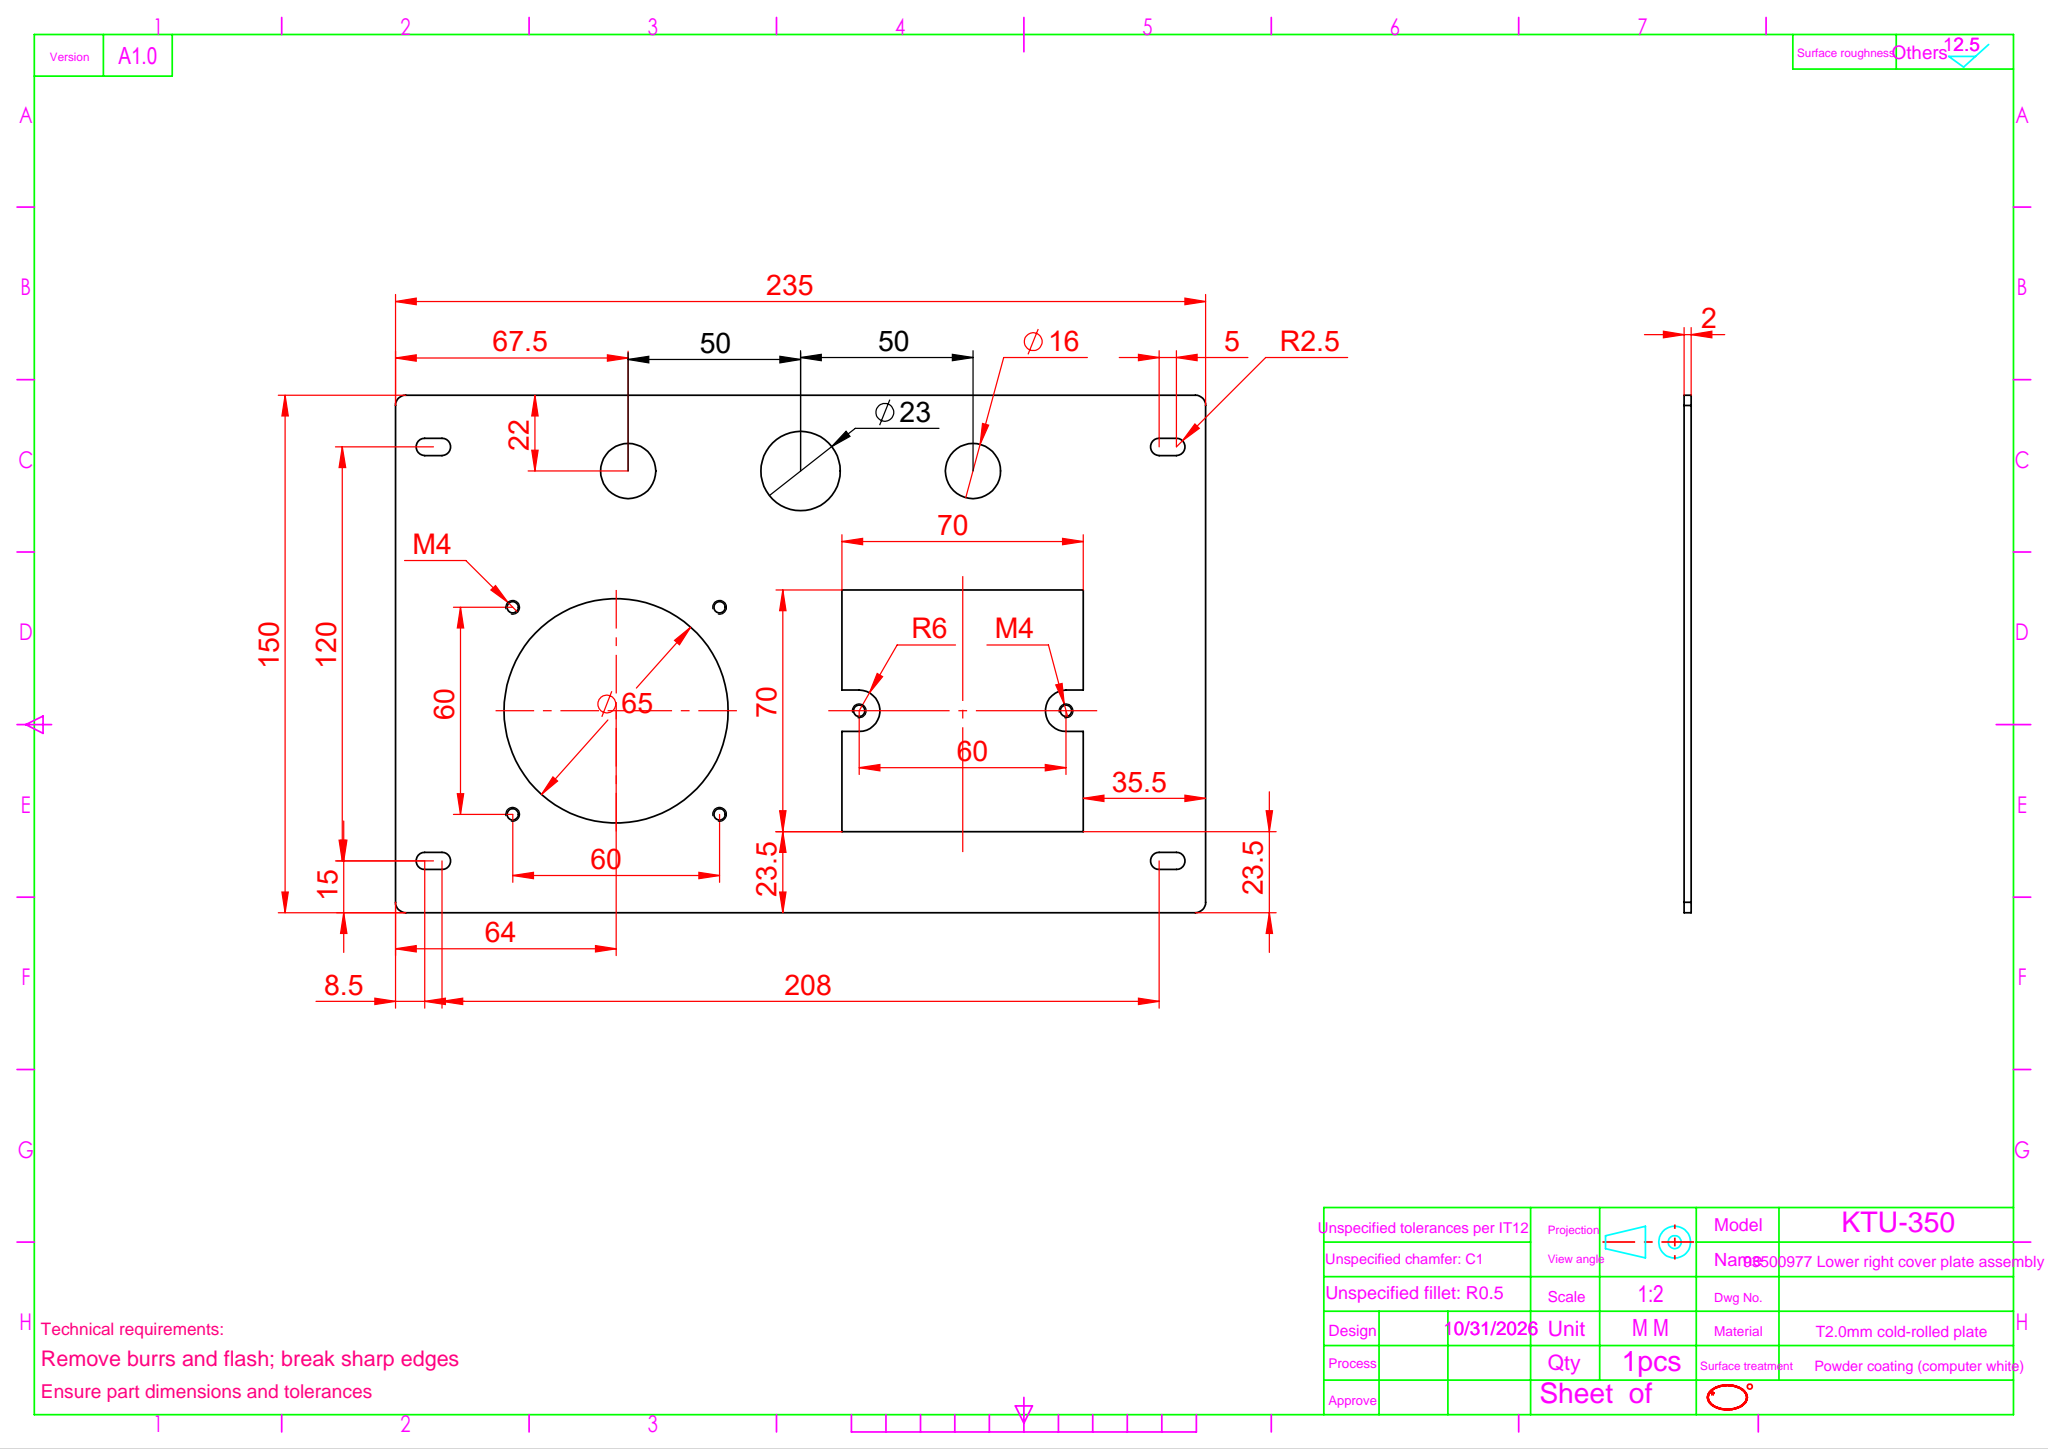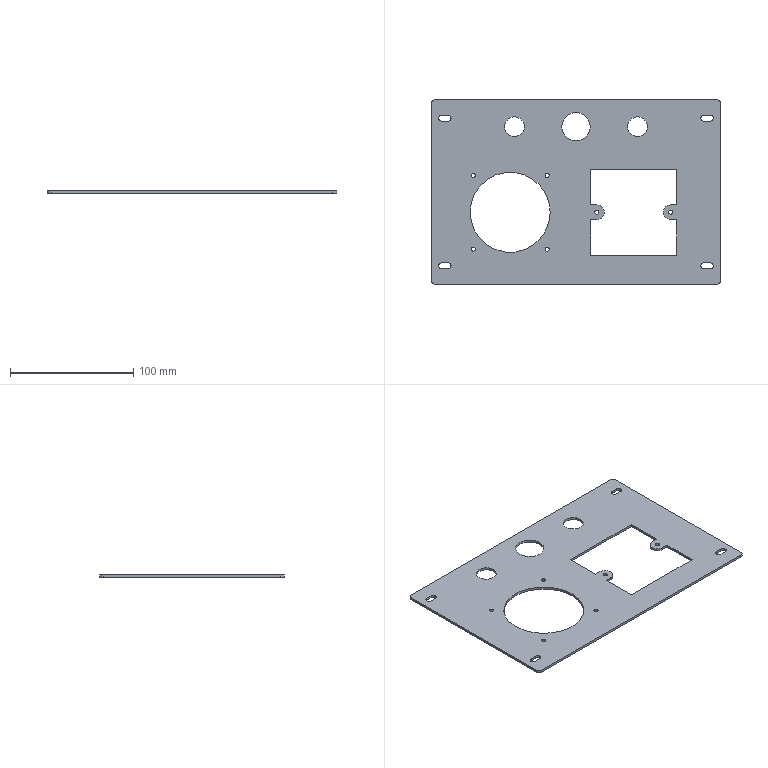Part | SolidWorks | features ICE 4, FlatPattern 1, HoleWzd 1, SMBaseFlange 1, SheetMetal 1 | 1 solid | 63 faces | box 235 x 150 x 2 mm | volume 52419 mm3 | cylinder 39 | plane 24 | commonest cylinder face diameters 3.3 x12 5 x12 6 x4 16 x4 12 x3 23 x2